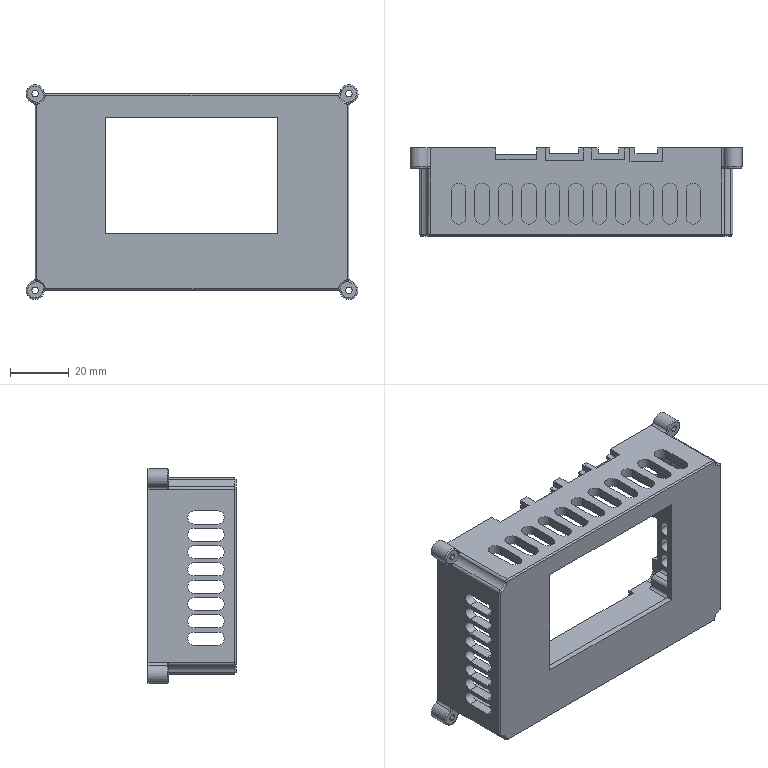Part | SolidWorks | features BaseBody 1, Chamfer 1, ICE 1 | 1 solid | 877 faces | box 113.2 x 30 x 73.2 mm | volume 35438 mm3 | plane 504 | spline 234 | cylinder 127 | cone 12 | commonest cylinder face diameters 2 x36 4.5 x32 5 x22 6.2 x10 3.6 x9 2.2 x8